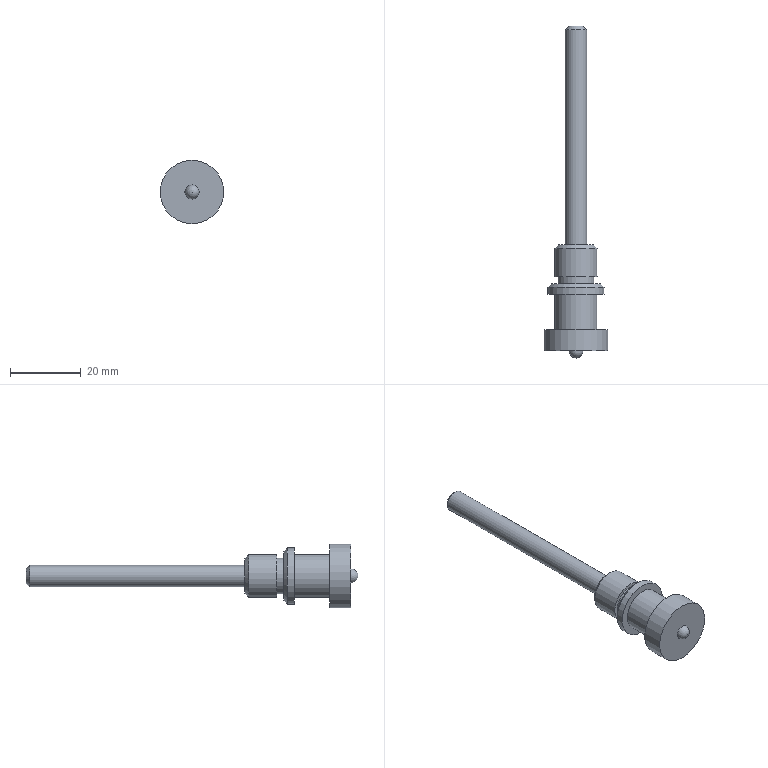Part | NX | features DATUM_CSYS 2, CHAMFER 1, SKETCH 1, SWP104 1, SYMBOLIC_THREAD 1 | 1 solid | 17 faces | box 18 x 94 x 18 mm | volume 6155 mm3 | plane 7 | cylinder 6 | cone 3 | sphere 1 | commonest cylinder face diameters 12 x2 6 x1 10 x1 16 x1 18 x1
STEP:
#1=CARTESIAN_POINT('',(0.,0.,-2.));
#2=VERTEX_POINT('',#1);
#3=CARTESIAN_POINT('',(0.,0.,0.));
#4=DIRECTION('',(0.,-1.,0.));
#5=DIRECTION('',(0.,0.,-1.));
#6=AXIS2_PLACEMENT_3D('',#3,#4,#5);
#7=CIRCLE('',#6,2.);
#8=EDGE_CURVE('',#2,#2,#7,.T.);
#9=ORIENTED_EDGE('',*,*,#8,.T.);
#10=EDGE_LOOP('',(#9));
#11=FACE_BOUND('',#10,.T.);
#12=CARTESIAN_POINT('',(0.,0.,0.));
#13=DIRECTION('',(0.,-1.,0.));
#14=DIRECTION('',(0.,0.,1.));
#15=AXIS2_PLACEMENT_3D('',#12,#13,#14);
#16=SPHERICAL_SURFACE('',#15,2.);
#17=ADVANCED_FACE('',(#11),#16,.T.);
#18=CARTESIAN_POINT('',(0.,92.,-2.));
#19=VERTEX_POINT('',#18);
#20=CARTESIAN_POINT('',(0.,92.,0.));
#21=DIRECTION('',(0.,-1.,0.));
#22=DIRECTION('',(0.,0.,-1.));
#23=AXIS2_PLACEMENT_3D('',#20,#21,#22);
#24=CIRCLE('',#23,2.);
#25=EDGE_CURVE('',#19,#19,#24,.T.);
#26=ORIENTED_EDGE('',*,*,#25,.F.);
#27=EDGE_LOOP('',(#26));
#28=FACE_BOUND('',#27,.T.);
#29=CARTESIAN_POINT('',(0.,92.,0.));
#30=DIRECTION('',(0.,-1.,0.));
#31=DIRECTION('',(0.,0.,-1.));
#32=AXIS2_PLACEMENT_3D('',#29,#30,#31);
#33=PLANE('',#32);
#34=ADVANCED_FACE('',(#28),#33,.F.);
#35=CARTESIAN_POINT('',(0.,91.,-3.));
#36=VERTEX_POINT('',#35);
#37=CARTESIAN_POINT('',(0.,91.,0.));
#38=DIRECTION('',(0.,-1.,0.));
#39=DIRECTION('',(0.,0.,-1.));
#40=AXIS2_PLACEMENT_3D('',#37,#38,#39);
#41=CIRCLE('',#40,3.);
#42=EDGE_CURVE('',#36,#36,#41,.T.);
#43=ORIENTED_EDGE('',*,*,#42,.F.);
#44=EDGE_LOOP('',(#43));
#45=FACE_BOUND('',#44,.T.);
#46=ORIENTED_EDGE('',*,*,#25,.T.);
#47=EDGE_LOOP('',(#46));
#48=FACE_BOUND('',#47,.T.);
#49=CARTESIAN_POINT('',(0.,92.,0.));
#50=DIRECTION('',(0.,-1.,0.));
#51=DIRECTION('',(0.,0.,-1.));
#52=AXIS2_PLACEMENT_3D('',#49,#50,#51);
#53=CONICAL_SURFACE('',#52,2.,0.7854);
#54=ADVANCED_FACE('',(#45,#48),#53,.T.);
#55=CARTESIAN_POINT('',(0.,30.,-3.));
#56=VERTEX_POINT('',#55);
#57=CARTESIAN_POINT('',(0.,30.,0.));
#58=DIRECTION('',(0.,-1.,0.));
#59=DIRECTION('',(0.,0.,-1.));
#60=AXIS2_PLACEMENT_3D('',#57,#58,#59);
#61=CIRCLE('',#60,3.);
#62=EDGE_CURVE('',#56,#56,#61,.T.);
#63=ORIENTED_EDGE('',*,*,#62,.F.);
#64=EDGE_LOOP('',(#63));
#65=FACE_BOUND('',#64,.T.);
#66=ORIENTED_EDGE('',*,*,#42,.T.);
#67=EDGE_LOOP('',(#66));
#68=FACE_BOUND('',#67,.T.);
#69=CARTESIAN_POINT('',(0.,-2.,0.));
#70=DIRECTION('',(0.,-1.,0.));
#71=DIRECTION('',(0.,0.,-1.));
#72=AXIS2_PLACEMENT_3D('',#69,#70,#71);
#73=CYLINDRICAL_SURFACE('',#72,3.);
#74=ADVANCED_FACE('',(#65,#68),#73,.T.);
#75=CARTESIAN_POINT('',(0.,30.,-5.));
#76=VERTEX_POINT('',#75);
#77=CARTESIAN_POINT('',(0.,30.,0.));
#78=DIRECTION('',(0.,-1.,0.));
#79=DIRECTION('',(0.,0.,-1.));
#80=AXIS2_PLACEMENT_3D('',#77,#78,#79);
#81=CIRCLE('',#80,5.);
#82=EDGE_CURVE('',#76,#76,#81,.F.);
#83=ORIENTED_EDGE('',*,*,#82,.T.);
#84=EDGE_LOOP('',(#83));
#85=FACE_BOUND('',#84,.T.);
#86=ORIENTED_EDGE('',*,*,#62,.T.);
#87=EDGE_LOOP('',(#86));
#88=FACE_BOUND('',#87,.T.);
#89=CARTESIAN_POINT('',(0.,30.,3.));
#90=DIRECTION('',(0.,-1.,0.));
#91=DIRECTION('',(0.,0.,-1.));
#92=AXIS2_PLACEMENT_3D('',#89,#90,#91);
#93=PLANE('',#92);
#94=ADVANCED_FACE('',(#85,#88),#93,.F.);
#95=CARTESIAN_POINT('',(0.,29.,-6.));
#96=VERTEX_POINT('',#95);
#97=CARTESIAN_POINT('',(0.,29.,0.));
#98=DIRECTION('',(0.,-1.,0.));
#99=DIRECTION('',(0.,0.,-1.));
#100=AXIS2_PLACEMENT_3D('',#97,#98,#99);
#101=CIRCLE('',#100,6.);
#102=EDGE_CURVE('',#96,#96,#101,.T.);
#103=ORIENTED_EDGE('',*,*,#102,.T.);
#104=EDGE_LOOP('',(#103));
#105=FACE_BOUND('',#104,.T.);
#106=CARTESIAN_POINT('',(0.,21.,-6.));
#107=VERTEX_POINT('',#106);
#108=CARTESIAN_POINT('',(0.,21.,0.));
#109=DIRECTION('',(0.,-1.,0.));
#110=DIRECTION('',(0.,0.,-1.));
#111=AXIS2_PLACEMENT_3D('',#108,#109,#110);
#112=CIRCLE('',#111,6.);
#113=EDGE_CURVE('',#107,#107,#112,.T.);
#114=ORIENTED_EDGE('',*,*,#113,.F.);
#115=EDGE_LOOP('',(#114));
#116=FACE_BOUND('',#115,.T.);
#117=CARTESIAN_POINT('',(0.,-2.,0.));
#118=DIRECTION('',(0.,-1.,0.));
#119=DIRECTION('',(0.,0.,-1.));
#120=AXIS2_PLACEMENT_3D('',#117,#118,#119);
#121=CYLINDRICAL_SURFACE('',#120,6.);
#122=ADVANCED_FACE('',(#105,#116),#121,.T.);
#123=CARTESIAN_POINT('',(0.,21.,-5.));
#124=VERTEX_POINT('',#123);
#125=CARTESIAN_POINT('',(0.,21.,0.));
#126=DIRECTION('',(0.,-1.,0.));
#127=DIRECTION('',(0.,0.,-1.));
#128=AXIS2_PLACEMENT_3D('',#125,#126,#127);
#129=CIRCLE('',#128,5.);
#130=EDGE_CURVE('',#124,#124,#129,.T.);
#131=ORIENTED_EDGE('',*,*,#130,.F.);
#132=EDGE_LOOP('',(#131));
#133=FACE_BOUND('',#132,.T.);
#134=ORIENTED_EDGE('',*,*,#113,.T.);
#135=EDGE_LOOP('',(#134));
#136=FACE_BOUND('',#135,.T.);
#137=CARTESIAN_POINT('',(0.,21.,6.));
#138=DIRECTION('',(0.,1.,0.));
#139=DIRECTION('',(0.,0.,1.));
#140=AXIS2_PLACEMENT_3D('',#137,#138,#139);
#141=PLANE('',#140);
#142=ADVANCED_FACE('',(#133,#136),#141,.F.);
#143=CARTESIAN_POINT('',(0.,19.,-5.));
#144=VERTEX_POINT('',#143);
#145=CARTESIAN_POINT('',(0.,19.,0.));
#146=DIRECTION('',(0.,-1.,0.));
#147=DIRECTION('',(0.,0.,-1.));
#148=AXIS2_PLACEMENT_3D('',#145,#146,#147);
#149=CIRCLE('',#148,5.);
#150=EDGE_CURVE('',#144,#144,#149,.T.);
#151=ORIENTED_EDGE('',*,*,#150,.F.);
#152=EDGE_LOOP('',(#151));
#153=FACE_BOUND('',#152,.T.);
#154=ORIENTED_EDGE('',*,*,#130,.T.);
#155=EDGE_LOOP('',(#154));
#156=FACE_BOUND('',#155,.T.);
#157=CARTESIAN_POINT('',(0.,-2.,0.));
#158=DIRECTION('',(0.,-1.,0.));
#159=DIRECTION('',(0.,0.,-1.));
#160=AXIS2_PLACEMENT_3D('',#157,#158,#159);
#161=CYLINDRICAL_SURFACE('',#160,5.);
#162=ADVANCED_FACE('',(#153,#156),#161,.T.);
#163=CARTESIAN_POINT('',(0.,19.,-7.));
#164=VERTEX_POINT('',#163);
#165=CARTESIAN_POINT('',(0.,19.,0.));
#166=DIRECTION('',(0.,-1.,0.));
#167=DIRECTION('',(0.,0.,-1.));
#168=AXIS2_PLACEMENT_3D('',#165,#166,#167);
#169=CIRCLE('',#168,7.);
#170=EDGE_CURVE('',#164,#164,#169,.T.);
#171=ORIENTED_EDGE('',*,*,#170,.F.);
#172=EDGE_LOOP('',(#171));
#173=FACE_BOUND('',#172,.T.);
#174=ORIENTED_EDGE('',*,*,#150,.T.);
#175=EDGE_LOOP('',(#174));
#176=FACE_BOUND('',#175,.T.);
#177=CARTESIAN_POINT('',(0.,19.,5.));
#178=DIRECTION('',(0.,-1.,0.));
#179=DIRECTION('',(0.,0.,-1.));
#180=AXIS2_PLACEMENT_3D('',#177,#178,#179);
#181=PLANE('',#180);
#182=ADVANCED_FACE('',(#173,#176),#181,.F.);
#183=CARTESIAN_POINT('',(0.,18.,-8.));
#184=VERTEX_POINT('',#183);
#185=CARTESIAN_POINT('',(0.,18.,0.));
#186=DIRECTION('',(0.,-1.,0.));
#187=DIRECTION('',(0.,0.,-1.));
#188=AXIS2_PLACEMENT_3D('',#185,#186,#187);
#189=CIRCLE('',#188,8.);
#190=EDGE_CURVE('',#184,#184,#189,.T.);
#191=ORIENTED_EDGE('',*,*,#190,.F.);
#192=EDGE_LOOP('',(#191));
#193=FACE_BOUND('',#192,.T.);
#194=ORIENTED_EDGE('',*,*,#170,.T.);
#195=EDGE_LOOP('',(#194));
#196=FACE_BOUND('',#195,.T.);
#197=CARTESIAN_POINT('',(0.,19.,0.));
#198=DIRECTION('',(0.,-1.,0.));
#199=DIRECTION('',(0.,0.,-1.));
#200=AXIS2_PLACEMENT_3D('',#197,#198,#199);
#201=CONICAL_SURFACE('',#200,7.,0.7854);
#202=ADVANCED_FACE('',(#193,#196),#201,.T.);
#203=CARTESIAN_POINT('',(0.,16.,-8.));
#204=VERTEX_POINT('',#203);
#205=CARTESIAN_POINT('',(0.,16.,0.));
#206=DIRECTION('',(0.,-1.,0.));
#207=DIRECTION('',(0.,0.,-1.));
#208=AXIS2_PLACEMENT_3D('',#205,#206,#207);
#209=CIRCLE('',#208,8.);
#210=EDGE_CURVE('',#204,#204,#209,.T.);
#211=ORIENTED_EDGE('',*,*,#210,.F.);
#212=EDGE_LOOP('',(#211));
#213=FACE_BOUND('',#212,.T.);
#214=ORIENTED_EDGE('',*,*,#190,.T.);
#215=EDGE_LOOP('',(#214));
#216=FACE_BOUND('',#215,.T.);
#217=CARTESIAN_POINT('',(0.,-2.,0.));
#218=DIRECTION('',(0.,-1.,0.));
#219=DIRECTION('',(0.,0.,-1.));
#220=AXIS2_PLACEMENT_3D('',#217,#218,#219);
#221=CYLINDRICAL_SURFACE('',#220,8.);
#222=ADVANCED_FACE('',(#213,#216),#221,.T.);
#223=CARTESIAN_POINT('',(0.,16.,-6.));
#224=VERTEX_POINT('',#223);
#225=CARTESIAN_POINT('',(0.,16.,0.));
#226=DIRECTION('',(0.,-1.,0.));
#227=DIRECTION('',(0.,0.,-1.));
#228=AXIS2_PLACEMENT_3D('',#225,#226,#227);
#229=CIRCLE('',#228,6.);
#230=EDGE_CURVE('',#224,#224,#229,.T.);
#231=ORIENTED_EDGE('',*,*,#230,.F.);
#232=EDGE_LOOP('',(#231));
#233=FACE_BOUND('',#232,.T.);
#234=ORIENTED_EDGE('',*,*,#210,.T.);
#235=EDGE_LOOP('',(#234));
#236=FACE_BOUND('',#235,.T.);
#237=CARTESIAN_POINT('',(0.,16.,8.));
#238=DIRECTION('',(0.,1.,0.));
#239=DIRECTION('',(0.,0.,1.));
#240=AXIS2_PLACEMENT_3D('',#237,#238,#239);
#241=PLANE('',#240);
#242=ADVANCED_FACE('',(#233,#236),#241,.F.);
#243=CARTESIAN_POINT('',(0.,6.,-6.));
#244=VERTEX_POINT('',#243);
#245=CARTESIAN_POINT('',(0.,6.,0.));
#246=DIRECTION('',(0.,-1.,0.));
#247=DIRECTION('',(0.,0.,-1.));
#248=AXIS2_PLACEMENT_3D('',#245,#246,#247);
#249=CIRCLE('',#248,6.);
#250=EDGE_CURVE('',#244,#244,#249,.T.);
#251=ORIENTED_EDGE('',*,*,#250,.F.);
#252=EDGE_LOOP('',(#251));
#253=FACE_BOUND('',#252,.T.);
#254=ORIENTED_EDGE('',*,*,#230,.T.);
#255=EDGE_LOOP('',(#254));
#256=FACE_BOUND('',#255,.T.);
#257=CARTESIAN_POINT('',(0.,-2.,0.));
#258=DIRECTION('',(0.,-1.,0.));
#259=DIRECTION('',(0.,0.,-1.));
#260=AXIS2_PLACEMENT_3D('',#257,#258,#259);
#261=CYLINDRICAL_SURFACE('',#260,6.);
#262=ADVANCED_FACE('',(#253,#256),#261,.T.);
#263=CARTESIAN_POINT('',(0.,6.,-9.));
#264=VERTEX_POINT('',#263);
#265=CARTESIAN_POINT('',(0.,6.,0.));
#266=DIRECTION('',(0.,-1.,0.));
#267=DIRECTION('',(0.,0.,-1.));
#268=AXIS2_PLACEMENT_3D('',#265,#266,#267);
#269=CIRCLE('',#268,9.);
#270=EDGE_CURVE('',#264,#264,#269,.T.);
#271=ORIENTED_EDGE('',*,*,#270,.F.);
#272=EDGE_LOOP('',(#271));
#273=FACE_BOUND('',#272,.T.);
#274=ORIENTED_EDGE('',*,*,#250,.T.);
#275=EDGE_LOOP('',(#274));
#276=FACE_BOUND('',#275,.T.);
#277=CARTESIAN_POINT('',(0.,6.,6.));
#278=DIRECTION('',(0.,-1.,0.));
#279=DIRECTION('',(0.,0.,-1.));
#280=AXIS2_PLACEMENT_3D('',#277,#278,#279);
#281=PLANE('',#280);
#282=ADVANCED_FACE('',(#273,#276),#281,.F.);
#283=CARTESIAN_POINT('',(0.,0.,-9.));
#284=VERTEX_POINT('',#283);
#285=CARTESIAN_POINT('',(0.,0.,0.));
#286=DIRECTION('',(0.,-1.,0.));
#287=DIRECTION('',(0.,0.,-1.));
#288=AXIS2_PLACEMENT_3D('',#285,#286,#287);
#289=CIRCLE('',#288,9.);
#290=EDGE_CURVE('',#284,#284,#289,.T.);
#291=ORIENTED_EDGE('',*,*,#290,.F.);
#292=EDGE_LOOP('',(#291));
#293=FACE_BOUND('',#292,.T.);
#294=ORIENTED_EDGE('',*,*,#270,.T.);
#295=EDGE_LOOP('',(#294));
#296=FACE_BOUND('',#295,.T.);
#297=CARTESIAN_POINT('',(0.,-2.,0.));
#298=DIRECTION('',(0.,-1.,0.));
#299=DIRECTION('',(0.,0.,-1.));
#300=AXIS2_PLACEMENT_3D('',#297,#298,#299);
#301=CYLINDRICAL_SURFACE('',#300,9.);
#302=ADVANCED_FACE('',(#293,#296),#301,.T.);
#303=ORIENTED_EDGE('',*,*,#8,.F.);
#304=EDGE_LOOP('',(#303));
#305=FACE_BOUND('',#304,.T.);
#306=ORIENTED_EDGE('',*,*,#290,.T.);
#307=EDGE_LOOP('',(#306));
#308=FACE_BOUND('',#307,.T.);
#309=CARTESIAN_POINT('',(0.,0.,9.));
#310=DIRECTION('',(0.,1.,0.));
#311=DIRECTION('',(0.,0.,1.));
#312=AXIS2_PLACEMENT_3D('',#309,#310,#311);
#313=PLANE('',#312);
#314=ADVANCED_FACE('',(#305,#308),#313,.F.);
#315=ORIENTED_EDGE('',*,*,#82,.F.);
#316=EDGE_LOOP('',(#315));
#317=FACE_BOUND('',#316,.T.);
#318=ORIENTED_EDGE('',*,*,#102,.F.);
#319=EDGE_LOOP('',(#318));
#320=FACE_BOUND('',#319,.T.);
#321=CARTESIAN_POINT('',(0.,29.,0.));
#322=DIRECTION('',(0.,-1.,0.));
#323=DIRECTION('',(0.,0.,-1.));
#324=AXIS2_PLACEMENT_3D('',#321,#322,#323);
#325=CONICAL_SURFACE('',#324,6.,0.7854);
#326=ADVANCED_FACE('',(#317,#320),#325,.T.);
#327=CLOSED_SHELL('',(#17,#34,#54,#74,#94,#122,#142,#162,#182,#202,#222,#242,#262,#282,#302,#314,#326));
#328=MANIFOLD_SOLID_BREP('',#327);
#329=(LENGTH_UNIT()NAMED_UNIT(*)SI_UNIT(.MILLI.,.METRE.));
#330=UNCERTAINTY_MEASURE_WITH_UNIT(LENGTH_MEASURE(0.00001),#329,'','');
#331=(NAMED_UNIT(*)PLANE_ANGLE_UNIT()SI_UNIT($,.RADIAN.));
#332=(NAMED_UNIT(*)SI_UNIT($,.STERADIAN.)SOLID_ANGLE_UNIT());
#333=(GEOMETRIC_REPRESENTATION_CONTEXT(3)GLOBAL_UNCERTAINTY_ASSIGNED_CONTEXT((#330))GLOBAL_UNIT_ASSIGNED_CONTEXT((#329,#331,#332))REPRESENTATION_CONTEXT('',''));
#334=ADVANCED_BREP_SHAPE_REPRESENTATION('',(#328),#333);